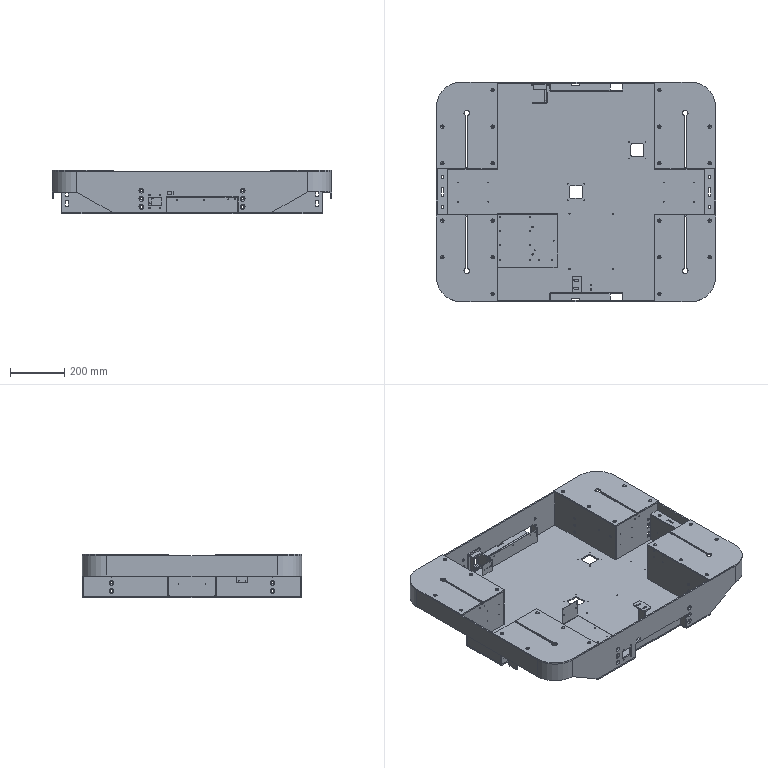Part | NX | features BREP 26 | 37 solids | 717 faces | box 1030 x 810 x 160 mm | volume 7743384 mm3 | plane 392 | cylinder 277 | cone 48 | commonest cylinder face diameters 4 x36 10 x35 9 x28 2.5 x24 6.5 x24 3.4 x22